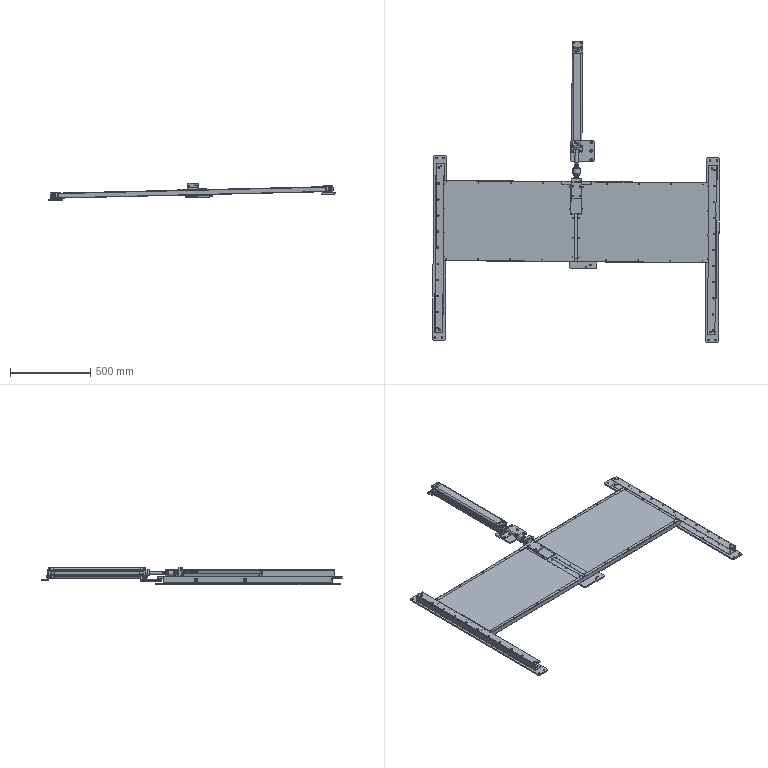Part | NX | features BREP 26 | 81 solids | 3784 faces | volume 6780207 mm3 | cylinder 1105 | plane 1031 | cone 688 | sphere 674 | torus 270 | spline 16 | commonest cylinder face diameters 10 x154 5.5 x112 1 x104 23.4 x64 4 x52 4.5 x48